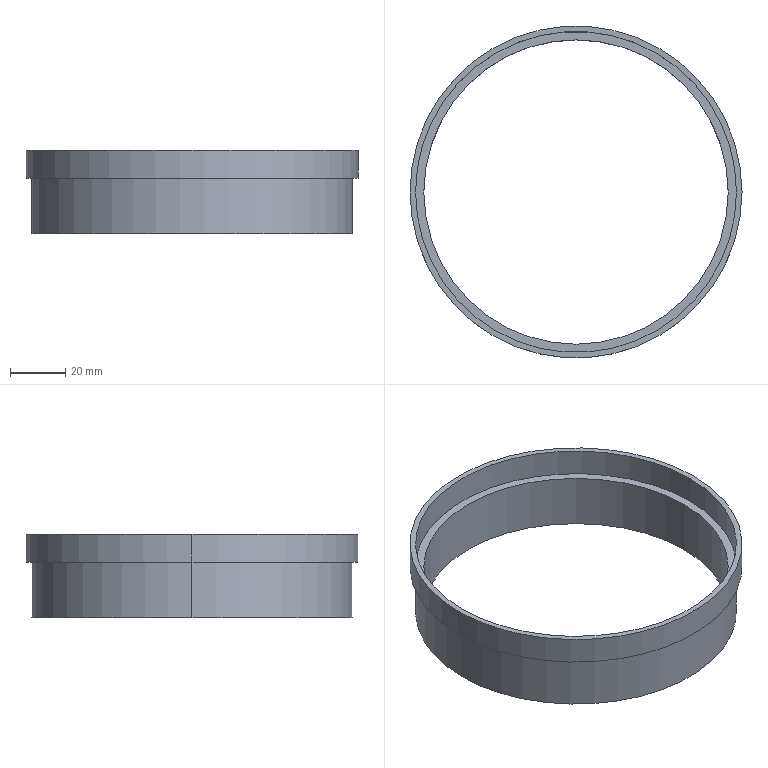Part | SolidWorks | features Extrusion 1, ICE 1 | 2 solids | 12 faces | box 120 x 120 x 30 mm | volume 28714 mm3 | cylinder 8 | plane 4 | commonest cylinder face diameters 116 x4 110 x2 120 x2
STEP:
#1=CARTESIAN_POINT('',(-55.,0.,20.));
#2=VERTEX_POINT('',#1);
#3=CARTESIAN_POINT('',(55.,0.,20.));
#4=VERTEX_POINT('',#3);
#5=CARTESIAN_POINT('',(0.,0.,20.));
#6=DIRECTION('',(0.,0.,1.));
#7=DIRECTION('',(1.,0.,0.));
#8=AXIS2_PLACEMENT_3D('',#5,#6,#7);
#9=CIRCLE('',#8,55.);
#10=EDGE_CURVE('',#2,#4,#9,.T.);
#11=ORIENTED_EDGE('',*,*,#10,.T.);
#12=CARTESIAN_POINT('',(55.,0.,0.));
#13=VERTEX_POINT('',#12);
#14=CARTESIAN_POINT('',(55.,0.,20.));
#15=DIRECTION('',(0.,0.,-1.));
#16=VECTOR('',#15,1000.);
#17=LINE('',#14,#16);
#18=EDGE_CURVE('',#4,#13,#17,.T.);
#19=ORIENTED_EDGE('',*,*,#18,.T.);
#20=CARTESIAN_POINT('',(-55.,0.,0.));
#21=VERTEX_POINT('',#20);
#22=CARTESIAN_POINT('',(0.,0.,0.));
#23=DIRECTION('',(0.,0.,1.));
#24=DIRECTION('',(1.,0.,0.));
#25=AXIS2_PLACEMENT_3D('',#22,#23,#24);
#26=CIRCLE('',#25,55.);
#27=EDGE_CURVE('',#21,#13,#26,.T.);
#28=ORIENTED_EDGE('',*,*,#27,.F.);
#29=CARTESIAN_POINT('',(-55.,0.,20.));
#30=DIRECTION('',(0.,0.,-1.));
#31=VECTOR('',#30,1000.);
#32=LINE('',#29,#31);
#33=EDGE_CURVE('',#2,#21,#32,.T.);
#34=ORIENTED_EDGE('',*,*,#33,.F.);
#35=EDGE_LOOP('',(#11,#19,#28,#34));
#36=FACE_OUTER_BOUND('',#35,.T.);
#37=CARTESIAN_POINT('',(0.,0.,20.));
#38=DIRECTION('',(0.,0.,-1.));
#39=DIRECTION('',(-1.,0.,0.));
#40=AXIS2_PLACEMENT_3D('',#37,#38,#39);
#41=CYLINDRICAL_SURFACE('',#40,55.);
#42=ADVANCED_FACE('',(#36),#41,.F.);
#43=CARTESIAN_POINT('',(58.,0.,20.));
#44=VERTEX_POINT('',#43);
#45=CARTESIAN_POINT('',(-58.,0.,20.));
#46=VERTEX_POINT('',#45);
#47=CARTESIAN_POINT('',(0.,0.,20.));
#48=DIRECTION('',(0.,0.,1.));
#49=DIRECTION('',(1.,0.,0.));
#50=AXIS2_PLACEMENT_3D('',#47,#48,#49);
#51=CIRCLE('',#50,58.);
#52=EDGE_CURVE('',#44,#46,#51,.T.);
#53=ORIENTED_EDGE('',*,*,#52,.F.);
#54=CARTESIAN_POINT('',(58.,0.,0.));
#55=VERTEX_POINT('',#54);
#56=CARTESIAN_POINT('',(58.,0.,20.));
#57=DIRECTION('',(0.,0.,-1.));
#58=VECTOR('',#57,1000.);
#59=LINE('',#56,#58);
#60=EDGE_CURVE('',#44,#55,#59,.T.);
#61=ORIENTED_EDGE('',*,*,#60,.T.);
#62=CARTESIAN_POINT('',(-58.,0.,0.));
#63=VERTEX_POINT('',#62);
#64=CARTESIAN_POINT('',(0.,0.,0.));
#65=DIRECTION('',(0.,0.,1.));
#66=DIRECTION('',(1.,0.,0.));
#67=AXIS2_PLACEMENT_3D('',#64,#65,#66);
#68=CIRCLE('',#67,58.);
#69=EDGE_CURVE('',#55,#63,#68,.T.);
#70=ORIENTED_EDGE('',*,*,#69,.T.);
#71=CARTESIAN_POINT('',(-58.,0.,20.));
#72=DIRECTION('',(0.,0.,-1.));
#73=VECTOR('',#72,1000.);
#74=LINE('',#71,#73);
#75=EDGE_CURVE('',#46,#63,#74,.T.);
#76=ORIENTED_EDGE('',*,*,#75,.F.);
#77=EDGE_LOOP('',(#53,#61,#70,#76));
#78=FACE_OUTER_BOUND('',#77,.T.);
#79=CARTESIAN_POINT('',(0.,0.,20.));
#80=DIRECTION('',(0.,0.,-1.));
#81=DIRECTION('',(-1.,0.,0.));
#82=AXIS2_PLACEMENT_3D('',#79,#80,#81);
#83=CYLINDRICAL_SURFACE('',#82,58.);
#84=ADVANCED_FACE('',(#78),#83,.T.);
#85=CARTESIAN_POINT('',(0.,0.,20.));
#86=DIRECTION('',(0.,0.,1.));
#87=DIRECTION('',(1.,0.,0.));
#88=AXIS2_PLACEMENT_3D('',#85,#86,#87);
#89=CIRCLE('',#88,58.);
#90=EDGE_CURVE('',#46,#44,#89,.T.);
#91=ORIENTED_EDGE('',*,*,#90,.T.);
#92=ORIENTED_EDGE('',*,*,#52,.T.);
#93=EDGE_LOOP('',(#91,#92));
#94=FACE_OUTER_BOUND('',#93,.T.);
#95=ORIENTED_EDGE('',*,*,#10,.F.);
#96=CARTESIAN_POINT('',(0.,0.,20.));
#97=DIRECTION('',(0.,0.,1.));
#98=DIRECTION('',(1.,0.,0.));
#99=AXIS2_PLACEMENT_3D('',#96,#97,#98);
#100=CIRCLE('',#99,55.);
#101=EDGE_CURVE('',#4,#2,#100,.T.);
#102=ORIENTED_EDGE('',*,*,#101,.F.);
#103=EDGE_LOOP('',(#95,#102));
#104=FACE_BOUND('',#103,.T.);
#105=CARTESIAN_POINT('',(0.,0.,20.));
#106=DIRECTION('',(0.,0.,1.));
#107=DIRECTION('',(1.,0.,0.));
#108=AXIS2_PLACEMENT_3D('',#105,#106,#107);
#109=PLANE('',#108);
#110=ADVANCED_FACE('',(#94,#104),#109,.T.);
#111=CARTESIAN_POINT('',(0.,0.,0.));
#112=DIRECTION('',(0.,0.,1.));
#113=DIRECTION('',(1.,0.,0.));
#114=AXIS2_PLACEMENT_3D('',#111,#112,#113);
#115=CIRCLE('',#114,58.);
#116=EDGE_CURVE('',#63,#55,#115,.T.);
#117=ORIENTED_EDGE('',*,*,#116,.F.);
#118=ORIENTED_EDGE('',*,*,#69,.F.);
#119=EDGE_LOOP('',(#117,#118));
#120=FACE_OUTER_BOUND('',#119,.T.);
#121=ORIENTED_EDGE('',*,*,#27,.T.);
#122=CARTESIAN_POINT('',(0.,0.,0.));
#123=DIRECTION('',(0.,0.,1.));
#124=DIRECTION('',(1.,0.,0.));
#125=AXIS2_PLACEMENT_3D('',#122,#123,#124);
#126=CIRCLE('',#125,55.);
#127=EDGE_CURVE('',#13,#21,#126,.T.);
#128=ORIENTED_EDGE('',*,*,#127,.T.);
#129=EDGE_LOOP('',(#121,#128));
#130=FACE_BOUND('',#129,.T.);
#131=CARTESIAN_POINT('',(0.,0.,0.));
#132=DIRECTION('',(0.,0.,1.));
#133=DIRECTION('',(1.,0.,0.));
#134=AXIS2_PLACEMENT_3D('',#131,#132,#133);
#135=PLANE('',#134);
#136=ADVANCED_FACE('',(#120,#130),#135,.F.);
#137=ORIENTED_EDGE('',*,*,#60,.F.);
#138=ORIENTED_EDGE('',*,*,#90,.F.);
#139=ORIENTED_EDGE('',*,*,#75,.T.);
#140=ORIENTED_EDGE('',*,*,#116,.T.);
#141=EDGE_LOOP('',(#137,#138,#139,#140));
#142=FACE_OUTER_BOUND('',#141,.T.);
#143=CARTESIAN_POINT('',(0.,0.,20.));
#144=DIRECTION('',(0.,0.,-1.));
#145=DIRECTION('',(-1.,0.,0.));
#146=AXIS2_PLACEMENT_3D('',#143,#144,#145);
#147=CYLINDRICAL_SURFACE('',#146,58.);
#148=ADVANCED_FACE('',(#142),#147,.T.);
#149=ORIENTED_EDGE('',*,*,#18,.F.);
#150=ORIENTED_EDGE('',*,*,#101,.T.);
#151=ORIENTED_EDGE('',*,*,#33,.T.);
#152=ORIENTED_EDGE('',*,*,#127,.F.);
#153=EDGE_LOOP('',(#149,#150,#151,#152));
#154=FACE_OUTER_BOUND('',#153,.T.);
#155=CARTESIAN_POINT('',(0.,0.,20.));
#156=DIRECTION('',(0.,0.,-1.));
#157=DIRECTION('',(-1.,0.,0.));
#158=AXIS2_PLACEMENT_3D('',#155,#156,#157);
#159=CYLINDRICAL_SURFACE('',#158,55.);
#160=ADVANCED_FACE('',(#154),#159,.F.);
#161=CLOSED_SHELL('',(#42,#84,#110,#136,#148,#160));
#162=MANIFOLD_SOLID_BREP('',#161);
#163=CARTESIAN_POINT('',(-58.,0.,30.));
#164=VERTEX_POINT('',#163);
#165=CARTESIAN_POINT('',(58.,0.,30.));
#166=VERTEX_POINT('',#165);
#167=CARTESIAN_POINT('',(0.,0.,30.));
#168=DIRECTION('',(0.,0.,1.));
#169=DIRECTION('',(1.,0.,0.));
#170=AXIS2_PLACEMENT_3D('',#167,#168,#169);
#171=CIRCLE('',#170,58.);
#172=EDGE_CURVE('',#164,#166,#171,.T.);
#173=ORIENTED_EDGE('',*,*,#172,.T.);
#174=CARTESIAN_POINT('',(58.,0.,20.));
#175=VERTEX_POINT('',#174);
#176=CARTESIAN_POINT('',(58.,0.,30.));
#177=DIRECTION('',(0.,0.,-1.));
#178=VECTOR('',#177,1000.);
#179=LINE('',#176,#178);
#180=EDGE_CURVE('',#166,#175,#179,.T.);
#181=ORIENTED_EDGE('',*,*,#180,.T.);
#182=CARTESIAN_POINT('',(-58.,0.,20.));
#183=VERTEX_POINT('',#182);
#184=CARTESIAN_POINT('',(0.,0.,20.));
#185=DIRECTION('',(0.,0.,1.));
#186=DIRECTION('',(1.,0.,0.));
#187=AXIS2_PLACEMENT_3D('',#184,#185,#186);
#188=CIRCLE('',#187,58.);
#189=EDGE_CURVE('',#183,#175,#188,.T.);
#190=ORIENTED_EDGE('',*,*,#189,.F.);
#191=CARTESIAN_POINT('',(-58.,0.,30.));
#192=DIRECTION('',(0.,0.,-1.));
#193=VECTOR('',#192,1000.);
#194=LINE('',#191,#193);
#195=EDGE_CURVE('',#164,#183,#194,.T.);
#196=ORIENTED_EDGE('',*,*,#195,.F.);
#197=EDGE_LOOP('',(#173,#181,#190,#196));
#198=FACE_OUTER_BOUND('',#197,.T.);
#199=CARTESIAN_POINT('',(0.,0.,30.));
#200=DIRECTION('',(0.,0.,-1.));
#201=DIRECTION('',(-1.,0.,0.));
#202=AXIS2_PLACEMENT_3D('',#199,#200,#201);
#203=CYLINDRICAL_SURFACE('',#202,58.);
#204=ADVANCED_FACE('',(#198),#203,.F.);
#205=CARTESIAN_POINT('',(60.,0.,30.));
#206=VERTEX_POINT('',#205);
#207=CARTESIAN_POINT('',(-60.,0.,30.));
#208=VERTEX_POINT('',#207);
#209=CARTESIAN_POINT('',(0.,0.,30.));
#210=DIRECTION('',(0.,0.,1.));
#211=DIRECTION('',(1.,0.,0.));
#212=AXIS2_PLACEMENT_3D('',#209,#210,#211);
#213=CIRCLE('',#212,60.);
#214=EDGE_CURVE('',#206,#208,#213,.T.);
#215=ORIENTED_EDGE('',*,*,#214,.F.);
#216=CARTESIAN_POINT('',(60.,0.,20.));
#217=VERTEX_POINT('',#216);
#218=CARTESIAN_POINT('',(60.,0.,30.));
#219=DIRECTION('',(0.,0.,-1.));
#220=VECTOR('',#219,1000.);
#221=LINE('',#218,#220);
#222=EDGE_CURVE('',#206,#217,#221,.T.);
#223=ORIENTED_EDGE('',*,*,#222,.T.);
#224=CARTESIAN_POINT('',(-60.,0.,20.));
#225=VERTEX_POINT('',#224);
#226=CARTESIAN_POINT('',(0.,0.,20.));
#227=DIRECTION('',(0.,0.,1.));
#228=DIRECTION('',(1.,0.,0.));
#229=AXIS2_PLACEMENT_3D('',#226,#227,#228);
#230=CIRCLE('',#229,60.);
#231=EDGE_CURVE('',#217,#225,#230,.T.);
#232=ORIENTED_EDGE('',*,*,#231,.T.);
#233=CARTESIAN_POINT('',(-60.,0.,30.));
#234=DIRECTION('',(0.,0.,-1.));
#235=VECTOR('',#234,1000.);
#236=LINE('',#233,#235);
#237=EDGE_CURVE('',#208,#225,#236,.T.);
#238=ORIENTED_EDGE('',*,*,#237,.F.);
#239=EDGE_LOOP('',(#215,#223,#232,#238));
#240=FACE_OUTER_BOUND('',#239,.T.);
#241=CARTESIAN_POINT('',(0.,0.,30.));
#242=DIRECTION('',(0.,0.,-1.));
#243=DIRECTION('',(-1.,0.,0.));
#244=AXIS2_PLACEMENT_3D('',#241,#242,#243);
#245=CYLINDRICAL_SURFACE('',#244,60.);
#246=ADVANCED_FACE('',(#240),#245,.T.);
#247=CARTESIAN_POINT('',(0.,0.,30.));
#248=DIRECTION('',(0.,0.,1.));
#249=DIRECTION('',(1.,0.,0.));
#250=AXIS2_PLACEMENT_3D('',#247,#248,#249);
#251=CIRCLE('',#250,60.);
#252=EDGE_CURVE('',#208,#206,#251,.T.);
#253=ORIENTED_EDGE('',*,*,#252,.T.);
#254=ORIENTED_EDGE('',*,*,#214,.T.);
#255=EDGE_LOOP('',(#253,#254));
#256=FACE_OUTER_BOUND('',#255,.T.);
#257=ORIENTED_EDGE('',*,*,#172,.F.);
#258=CARTESIAN_POINT('',(0.,0.,30.));
#259=DIRECTION('',(0.,0.,1.));
#260=DIRECTION('',(1.,0.,0.));
#261=AXIS2_PLACEMENT_3D('',#258,#259,#260);
#262=CIRCLE('',#261,58.);
#263=EDGE_CURVE('',#166,#164,#262,.T.);
#264=ORIENTED_EDGE('',*,*,#263,.F.);
#265=EDGE_LOOP('',(#257,#264));
#266=FACE_BOUND('',#265,.T.);
#267=CARTESIAN_POINT('',(0.,0.,30.));
#268=DIRECTION('',(0.,0.,1.));
#269=DIRECTION('',(1.,0.,0.));
#270=AXIS2_PLACEMENT_3D('',#267,#268,#269);
#271=PLANE('',#270);
#272=ADVANCED_FACE('',(#256,#266),#271,.T.);
#273=CARTESIAN_POINT('',(0.,0.,20.));
#274=DIRECTION('',(0.,0.,1.));
#275=DIRECTION('',(1.,0.,0.));
#276=AXIS2_PLACEMENT_3D('',#273,#274,#275);
#277=CIRCLE('',#276,60.);
#278=EDGE_CURVE('',#225,#217,#277,.T.);
#279=ORIENTED_EDGE('',*,*,#278,.F.);
#280=ORIENTED_EDGE('',*,*,#231,.F.);
#281=EDGE_LOOP('',(#279,#280));
#282=FACE_OUTER_BOUND('',#281,.T.);
#283=ORIENTED_EDGE('',*,*,#189,.T.);
#284=CARTESIAN_POINT('',(0.,0.,20.));
#285=DIRECTION('',(0.,0.,1.));
#286=DIRECTION('',(1.,0.,0.));
#287=AXIS2_PLACEMENT_3D('',#284,#285,#286);
#288=CIRCLE('',#287,58.);
#289=EDGE_CURVE('',#175,#183,#288,.T.);
#290=ORIENTED_EDGE('',*,*,#289,.T.);
#291=EDGE_LOOP('',(#283,#290));
#292=FACE_BOUND('',#291,.T.);
#293=CARTESIAN_POINT('',(0.,0.,20.));
#294=DIRECTION('',(0.,0.,1.));
#295=DIRECTION('',(1.,0.,0.));
#296=AXIS2_PLACEMENT_3D('',#293,#294,#295);
#297=PLANE('',#296);
#298=ADVANCED_FACE('',(#282,#292),#297,.F.);
#299=ORIENTED_EDGE('',*,*,#222,.F.);
#300=ORIENTED_EDGE('',*,*,#252,.F.);
#301=ORIENTED_EDGE('',*,*,#237,.T.);
#302=ORIENTED_EDGE('',*,*,#278,.T.);
#303=EDGE_LOOP('',(#299,#300,#301,#302));
#304=FACE_OUTER_BOUND('',#303,.T.);
#305=CARTESIAN_POINT('',(0.,0.,30.));
#306=DIRECTION('',(0.,0.,-1.));
#307=DIRECTION('',(-1.,0.,0.));
#308=AXIS2_PLACEMENT_3D('',#305,#306,#307);
#309=CYLINDRICAL_SURFACE('',#308,60.);
#310=ADVANCED_FACE('',(#304),#309,.T.);
#311=ORIENTED_EDGE('',*,*,#180,.F.);
#312=ORIENTED_EDGE('',*,*,#263,.T.);
#313=ORIENTED_EDGE('',*,*,#195,.T.);
#314=ORIENTED_EDGE('',*,*,#289,.F.);
#315=EDGE_LOOP('',(#311,#312,#313,#314));
#316=FACE_OUTER_BOUND('',#315,.T.);
#317=CARTESIAN_POINT('',(0.,0.,30.));
#318=DIRECTION('',(0.,0.,-1.));
#319=DIRECTION('',(-1.,0.,0.));
#320=AXIS2_PLACEMENT_3D('',#317,#318,#319);
#321=CYLINDRICAL_SURFACE('',#320,58.);
#322=ADVANCED_FACE('',(#316),#321,.F.);
#323=CLOSED_SHELL('',(#204,#246,#272,#298,#310,#322));
#324=MANIFOLD_SOLID_BREP('',#323);
#325=CARTESIAN_POINT('',(0.,0.,0.));
#326=DIRECTION('',(0.,0.,1.));
#327=DIRECTION('',(1.,0.,0.));
#328=AXIS2_PLACEMENT_3D('',#325,#326,#327);
#329=(LENGTH_UNIT()NAMED_UNIT(*)SI_UNIT(.MILLI.,.METRE.));
#330=UNCERTAINTY_MEASURE_WITH_UNIT(LENGTH_MEASURE(0.00001),#329,'','');
#331=(NAMED_UNIT(*)PLANE_ANGLE_UNIT()SI_UNIT($,.RADIAN.));
#332=(NAMED_UNIT(*)SI_UNIT($,.STERADIAN.)SOLID_ANGLE_UNIT());
#333=(GEOMETRIC_REPRESENTATION_CONTEXT(3)GLOBAL_UNCERTAINTY_ASSIGNED_CONTEXT((#330))GLOBAL_UNIT_ASSIGNED_CONTEXT((#329,#331,#332))REPRESENTATION_CONTEXT('',''));
#334=ADVANCED_BREP_SHAPE_REPRESENTATION('',(#162,#324,#328),#333);